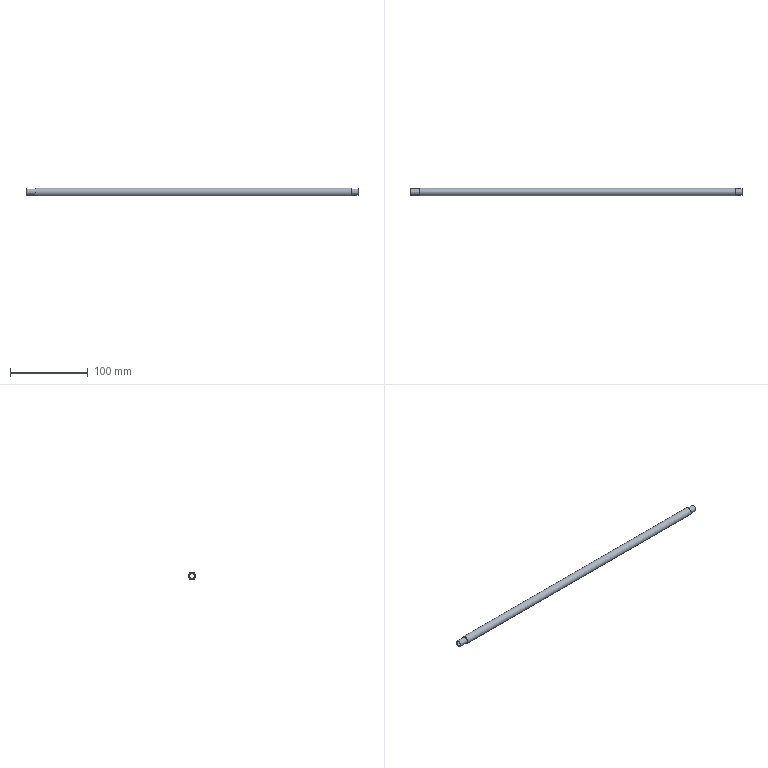Part | STEP file | 1-23.4 | 1 solid | 8 faces | box 427 x 10 x 10 mm | volume 20870 mm3 | cylinder 4 | plane 4 | commonest cylinder face diameters 8 x2 6 x1 10 x1
STEP:
#1=CARTESIAN_POINT('',(0.,0.,0.));
#2=DIRECTION('',(0.,0.,1.));
#3=DIRECTION('',(1.,0.,0.));
#4=AXIS2_PLACEMENT_3D('',#1,#2,#3);
#5=CARTESIAN_POINT('',(0.,5.,0.));
#6=VERTEX_POINT('',#5);
#7=CARTESIAN_POINT('',(-406.,5.,0.));
#8=VERTEX_POINT('',#7);
#9=CARTESIAN_POINT('',(0.,5.,0.));
#10=DIRECTION('',(-1.,0.,0.));
#11=VECTOR('',#10,1.);
#12=LINE('',#9,#11);
#13=CARTESIAN_POINT('',(0.,0.,0.));
#14=DIRECTION('',(-1.,0.,0.));
#15=DIRECTION('',(0.,1.,0.));
#16=AXIS2_PLACEMENT_3D('',#13,#14,#15);
#17=CYLINDRICAL_SURFACE('',#16,5.);
#18=CARTESIAN_POINT('',(6.283,0.));
#19=DIRECTION('',(0.,1.));
#20=VECTOR('',#19,1.);
#21=LINE('',#18,#20);
#22=(GEOMETRIC_REPRESENTATION_CONTEXT(2)PARAMETRIC_REPRESENTATION_CONTEXT()REPRESENTATION_CONTEXT('',''));
#23=DEFINITIONAL_REPRESENTATION('',(#21),#22);
#24=PCURVE('',#17,#23);
#25=CARTESIAN_POINT('',(0.,0.));
#26=DIRECTION('',(0.,1.));
#27=VECTOR('',#26,1.);
#28=LINE('',#25,#27);
#29=(GEOMETRIC_REPRESENTATION_CONTEXT(2)PARAMETRIC_REPRESENTATION_CONTEXT()REPRESENTATION_CONTEXT('',''));
#30=DEFINITIONAL_REPRESENTATION('',(#28),#29);
#31=PCURVE('',#17,#30);
#32=SEAM_CURVE('',#12,(#24,#31),.PCURVE_S1.);
#33=EDGE_CURVE('',#6,#8,#32,.T.);
#34=ORIENTED_EDGE('',*,*,#33,.T.);
#35=CARTESIAN_POINT('',(-406.,0.,0.));
#36=DIRECTION('',(1.,0.,0.));
#37=DIRECTION('',(0.,1.,0.));
#38=AXIS2_PLACEMENT_3D('',#35,#36,#37);
#39=CIRCLE('',#38,5.);
#40=CARTESIAN_POINT('',(6.283,406.));
#41=DIRECTION('',(-1.,0.));
#42=VECTOR('',#41,1.);
#43=LINE('',#40,#42);
#44=(GEOMETRIC_REPRESENTATION_CONTEXT(2)PARAMETRIC_REPRESENTATION_CONTEXT()REPRESENTATION_CONTEXT('',''));
#45=DEFINITIONAL_REPRESENTATION('',(#43),#44);
#46=PCURVE('',#17,#45);
#47=CARTESIAN_POINT('',(-406.,-1.34,0.));
#48=DIRECTION('',(1.,0.,0.));
#49=DIRECTION('',(0.,0.,-1.));
#50=AXIS2_PLACEMENT_3D('',#47,#48,#49);
#51=PLANE('',#50);
#52=CARTESIAN_POINT('',(0.,1.34));
#53=DIRECTION('',(0.,1.));
#54=AXIS2_PLACEMENT_2D('',#52,#53);
#55=CIRCLE('',#54,5.);
#56=(GEOMETRIC_REPRESENTATION_CONTEXT(2)PARAMETRIC_REPRESENTATION_CONTEXT()REPRESENTATION_CONTEXT('',''));
#57=DEFINITIONAL_REPRESENTATION('',(#55),#56);
#58=PCURVE('',#51,#57);
#59=SURFACE_CURVE('',#39,(#46,#58),.PCURVE_S1.);
#60=EDGE_CURVE('',#8,#8,#59,.T.);
#61=ORIENTED_EDGE('',*,*,#60,.T.);
#62=ORIENTED_EDGE('',*,*,#33,.F.);
#63=CARTESIAN_POINT('',(0.,0.,0.));
#64=DIRECTION('',(1.,0.,0.));
#65=DIRECTION('',(0.,1.,0.));
#66=AXIS2_PLACEMENT_3D('',#63,#64,#65);
#67=CIRCLE('',#66,5.);
#68=CARTESIAN_POINT('',(6.283,0.));
#69=DIRECTION('',(-1.,0.));
#70=VECTOR('',#69,1.);
#71=LINE('',#68,#70);
#72=(GEOMETRIC_REPRESENTATION_CONTEXT(2)PARAMETRIC_REPRESENTATION_CONTEXT()REPRESENTATION_CONTEXT('',''));
#73=DEFINITIONAL_REPRESENTATION('',(#71),#72);
#74=PCURVE('',#17,#73);
#75=CARTESIAN_POINT('',(0.,-1.34,0.));
#76=DIRECTION('',(1.,0.,0.));
#77=DIRECTION('',(0.,0.,-1.));
#78=AXIS2_PLACEMENT_3D('',#75,#76,#77);
#79=PLANE('',#78);
#80=CARTESIAN_POINT('',(0.,1.34));
#81=DIRECTION('',(0.,1.));
#82=AXIS2_PLACEMENT_2D('',#80,#81);
#83=CIRCLE('',#82,5.);
#84=(GEOMETRIC_REPRESENTATION_CONTEXT(2)PARAMETRIC_REPRESENTATION_CONTEXT()REPRESENTATION_CONTEXT('',''));
#85=DEFINITIONAL_REPRESENTATION('',(#83),#84);
#86=PCURVE('',#79,#85);
#87=SURFACE_CURVE('',#67,(#74,#86),.PCURVE_S1.);
#88=EDGE_CURVE('',#6,#6,#87,.T.);
#89=ORIENTED_EDGE('',*,*,#88,.F.);
#90=EDGE_LOOP('',(#34,#61,#62,#89));
#91=FACE_BOUND('',#90,.T.);
#92=ADVANCED_FACE('',(#91),#17,.T.);
#93=ORIENTED_EDGE('',*,*,#88,.T.);
#94=EDGE_LOOP('',(#93));
#95=FACE_BOUND('',#94,.T.);
#96=CARTESIAN_POINT('',(0.,4.,0.));
#97=VERTEX_POINT('',#96);
#98=CARTESIAN_POINT('',(0.,0.,0.));
#99=DIRECTION('',(1.,0.,0.));
#100=DIRECTION('',(0.,1.,0.));
#101=AXIS2_PLACEMENT_3D('',#98,#99,#100);
#102=CIRCLE('',#101,4.);
#103=CARTESIAN_POINT('',(0.,1.34));
#104=DIRECTION('',(0.,1.));
#105=AXIS2_PLACEMENT_2D('',#103,#104);
#106=CIRCLE('',#105,4.);
#107=(GEOMETRIC_REPRESENTATION_CONTEXT(2)PARAMETRIC_REPRESENTATION_CONTEXT()REPRESENTATION_CONTEXT('',''));
#108=DEFINITIONAL_REPRESENTATION('',(#106),#107);
#109=PCURVE('',#79,#108);
#110=CARTESIAN_POINT('',(0.,0.,0.));
#111=DIRECTION('',(1.,0.,0.));
#112=DIRECTION('',(0.,1.,0.));
#113=AXIS2_PLACEMENT_3D('',#110,#111,#112);
#114=CYLINDRICAL_SURFACE('',#113,4.);
#115=CARTESIAN_POINT('',(0.,0.));
#116=DIRECTION('',(1.,0.));
#117=VECTOR('',#116,1.);
#118=LINE('',#115,#117);
#119=(GEOMETRIC_REPRESENTATION_CONTEXT(2)PARAMETRIC_REPRESENTATION_CONTEXT()REPRESENTATION_CONTEXT('',''));
#120=DEFINITIONAL_REPRESENTATION('',(#118),#119);
#121=PCURVE('',#114,#120);
#122=SURFACE_CURVE('',#102,(#109,#121),.PCURVE_S1.);
#123=EDGE_CURVE('',#97,#97,#122,.T.);
#124=ORIENTED_EDGE('',*,*,#123,.F.);
#125=EDGE_LOOP('',(#124));
#126=FACE_BOUND('',#125,.T.);
#127=ADVANCED_FACE('',(#95,#126),#79,.T.);
#128=ORIENTED_EDGE('',*,*,#123,.T.);
#129=CARTESIAN_POINT('',(9.,4.,0.));
#130=VERTEX_POINT('',#129);
#131=CARTESIAN_POINT('',(0.,4.,0.));
#132=DIRECTION('',(1.,0.,0.));
#133=VECTOR('',#132,1.);
#134=LINE('',#131,#133);
#135=CARTESIAN_POINT('',(6.283,0.));
#136=DIRECTION('',(0.,1.));
#137=VECTOR('',#136,1.);
#138=LINE('',#135,#137);
#139=(GEOMETRIC_REPRESENTATION_CONTEXT(2)PARAMETRIC_REPRESENTATION_CONTEXT()REPRESENTATION_CONTEXT('',''));
#140=DEFINITIONAL_REPRESENTATION('',(#138),#139);
#141=PCURVE('',#114,#140);
#142=CARTESIAN_POINT('',(0.,0.));
#143=DIRECTION('',(0.,1.));
#144=VECTOR('',#143,1.);
#145=LINE('',#142,#144);
#146=(GEOMETRIC_REPRESENTATION_CONTEXT(2)PARAMETRIC_REPRESENTATION_CONTEXT()REPRESENTATION_CONTEXT('',''));
#147=DEFINITIONAL_REPRESENTATION('',(#145),#146);
#148=PCURVE('',#114,#147);
#149=SEAM_CURVE('',#134,(#141,#148),.PCURVE_S1.);
#150=EDGE_CURVE('',#97,#130,#149,.T.);
#151=ORIENTED_EDGE('',*,*,#150,.T.);
#152=CARTESIAN_POINT('',(9.,0.,0.));
#153=DIRECTION('',(1.,0.,0.));
#154=DIRECTION('',(0.,1.,0.));
#155=AXIS2_PLACEMENT_3D('',#152,#153,#154);
#156=CIRCLE('',#155,4.);
#157=CARTESIAN_POINT('',(0.,9.));
#158=DIRECTION('',(1.,0.));
#159=VECTOR('',#158,1.);
#160=LINE('',#157,#159);
#161=(GEOMETRIC_REPRESENTATION_CONTEXT(2)PARAMETRIC_REPRESENTATION_CONTEXT()REPRESENTATION_CONTEXT('',''));
#162=DEFINITIONAL_REPRESENTATION('',(#160),#161);
#163=PCURVE('',#114,#162);
#164=CARTESIAN_POINT('',(9.,-1.072,0.));
#165=DIRECTION('',(1.,0.,0.));
#166=DIRECTION('',(0.,0.,-1.));
#167=AXIS2_PLACEMENT_3D('',#164,#165,#166);
#168=PLANE('',#167);
#169=CARTESIAN_POINT('',(0.,1.072));
#170=DIRECTION('',(0.,1.));
#171=AXIS2_PLACEMENT_2D('',#169,#170);
#172=CIRCLE('',#171,4.);
#173=(GEOMETRIC_REPRESENTATION_CONTEXT(2)PARAMETRIC_REPRESENTATION_CONTEXT()REPRESENTATION_CONTEXT('',''));
#174=DEFINITIONAL_REPRESENTATION('',(#172),#173);
#175=PCURVE('',#168,#174);
#176=SURFACE_CURVE('',#156,(#163,#175),.PCURVE_S1.);
#177=EDGE_CURVE('',#130,#130,#176,.T.);
#178=ORIENTED_EDGE('',*,*,#177,.F.);
#179=ORIENTED_EDGE('',*,*,#150,.F.);
#180=EDGE_LOOP('',(#128,#151,#178,#179));
#181=FACE_BOUND('',#180,.T.);
#182=ADVANCED_FACE('',(#181),#114,.T.);
#183=ORIENTED_EDGE('',*,*,#60,.T.);
#184=EDGE_LOOP('',(#183));
#185=FACE_BOUND('',#184,.F.);
#186=CARTESIAN_POINT('',(-406.,-4.,0.));
#187=VERTEX_POINT('',#186);
#188=CARTESIAN_POINT('',(-406.,0.,0.));
#189=DIRECTION('',(-1.,0.,0.));
#190=DIRECTION('',(0.,-1.,0.));
#191=AXIS2_PLACEMENT_3D('',#188,#189,#190);
#192=CIRCLE('',#191,4.);
#193=CARTESIAN_POINT('',(0.,-2.66));
#194=CARTESIAN_POINT('',(-6.928,-2.66));
#195=CARTESIAN_POINT('',(-3.464,3.34));
#196=CARTESIAN_POINT('',(0.,9.34));
#197=CARTESIAN_POINT('',(3.464,3.34));
#198=CARTESIAN_POINT('',(6.928,-2.66));
#199=CARTESIAN_POINT('',(0.,-2.66));
#200=(BOUNDED_CURVE()B_SPLINE_CURVE(2,(#193,#194,#195,#196,#197,#198,#199),.UNSPECIFIED.,.T.,.F.)B_SPLINE_CURVE_WITH_KNOTS((1,2,2,2,2,1),(-2.094,0.,2.094,4.189,6.283,8.378),.UNSPECIFIED.)CURVE()GEOMETRIC_REPRESENTATION_ITEM()RATIONAL_B_SPLINE_CURVE((1.,0.5,1.,0.5,1.,0.5,1.))REPRESENTATION_ITEM(''));
#201=(GEOMETRIC_REPRESENTATION_CONTEXT(2)PARAMETRIC_REPRESENTATION_CONTEXT()REPRESENTATION_CONTEXT('',''));
#202=DEFINITIONAL_REPRESENTATION('',(#200),#201);
#203=PCURVE('',#51,#202);
#204=CARTESIAN_POINT('',(-406.,0.,0.));
#205=DIRECTION('',(-1.,0.,0.));
#206=DIRECTION('',(0.,-1.,0.));
#207=AXIS2_PLACEMENT_3D('',#204,#205,#206);
#208=CYLINDRICAL_SURFACE('',#207,4.);
#209=CARTESIAN_POINT('',(0.,0.));
#210=DIRECTION('',(1.,0.));
#211=VECTOR('',#210,1.);
#212=LINE('',#209,#211);
#213=(GEOMETRIC_REPRESENTATION_CONTEXT(2)PARAMETRIC_REPRESENTATION_CONTEXT()REPRESENTATION_CONTEXT('',''));
#214=DEFINITIONAL_REPRESENTATION('',(#212),#213);
#215=PCURVE('',#208,#214);
#216=SURFACE_CURVE('',#192,(#203,#215),.PCURVE_S1.);
#217=EDGE_CURVE('',#187,#187,#216,.T.);
#218=ORIENTED_EDGE('',*,*,#217,.T.);
#219=EDGE_LOOP('',(#218));
#220=FACE_BOUND('',#219,.F.);
#221=ADVANCED_FACE('',(#185,#220),#51,.F.);
#222=ORIENTED_EDGE('',*,*,#217,.T.);
#223=CARTESIAN_POINT('',(-418.,-4.,0.));
#224=VERTEX_POINT('',#223);
#225=CARTESIAN_POINT('',(-406.,-4.,0.));
#226=DIRECTION('',(-1.,0.,0.));
#227=VECTOR('',#226,1.);
#228=LINE('',#225,#227);
#229=CARTESIAN_POINT('',(6.283,0.));
#230=DIRECTION('',(0.,1.));
#231=VECTOR('',#230,1.);
#232=LINE('',#229,#231);
#233=(GEOMETRIC_REPRESENTATION_CONTEXT(2)PARAMETRIC_REPRESENTATION_CONTEXT()REPRESENTATION_CONTEXT('',''));
#234=DEFINITIONAL_REPRESENTATION('',(#232),#233);
#235=PCURVE('',#208,#234);
#236=CARTESIAN_POINT('',(0.,0.));
#237=DIRECTION('',(0.,1.));
#238=VECTOR('',#237,1.);
#239=LINE('',#236,#238);
#240=(GEOMETRIC_REPRESENTATION_CONTEXT(2)PARAMETRIC_REPRESENTATION_CONTEXT()REPRESENTATION_CONTEXT('',''));
#241=DEFINITIONAL_REPRESENTATION('',(#239),#240);
#242=PCURVE('',#208,#241);
#243=SEAM_CURVE('',#228,(#235,#242),.PCURVE_S1.);
#244=EDGE_CURVE('',#187,#224,#243,.T.);
#245=ORIENTED_EDGE('',*,*,#244,.T.);
#246=CARTESIAN_POINT('',(-418.,0.,0.));
#247=DIRECTION('',(-1.,0.,0.));
#248=DIRECTION('',(0.,-1.,0.));
#249=AXIS2_PLACEMENT_3D('',#246,#247,#248);
#250=CIRCLE('',#249,4.);
#251=CARTESIAN_POINT('',(0.,12.));
#252=DIRECTION('',(1.,0.));
#253=VECTOR('',#252,1.);
#254=LINE('',#251,#253);
#255=(GEOMETRIC_REPRESENTATION_CONTEXT(2)PARAMETRIC_REPRESENTATION_CONTEXT()REPRESENTATION_CONTEXT('',''));
#256=DEFINITIONAL_REPRESENTATION('',(#254),#255);
#257=PCURVE('',#208,#256);
#258=CARTESIAN_POINT('',(-418.,1.072,0.));
#259=DIRECTION('',(-1.,0.,0.));
#260=DIRECTION('',(0.,-1.,0.));
#261=AXIS2_PLACEMENT_3D('',#258,#259,#260);
#262=PLANE('',#261);
#263=CARTESIAN_POINT('',(1.072,0.));
#264=DIRECTION('',(1.,0.));
#265=AXIS2_PLACEMENT_2D('',#263,#264);
#266=CIRCLE('',#265,4.);
#267=(GEOMETRIC_REPRESENTATION_CONTEXT(2)PARAMETRIC_REPRESENTATION_CONTEXT()REPRESENTATION_CONTEXT('',''));
#268=DEFINITIONAL_REPRESENTATION('',(#266),#267);
#269=PCURVE('',#262,#268);
#270=SURFACE_CURVE('',#250,(#257,#269),.PCURVE_S1.);
#271=EDGE_CURVE('',#224,#224,#270,.T.);
#272=ORIENTED_EDGE('',*,*,#271,.F.);
#273=ORIENTED_EDGE('',*,*,#244,.F.);
#274=EDGE_LOOP('',(#222,#245,#272,#273));
#275=FACE_BOUND('',#274,.T.);
#276=ADVANCED_FACE('',(#275),#208,.T.);
#277=ORIENTED_EDGE('',*,*,#177,.T.);
#278=EDGE_LOOP('',(#277));
#279=FACE_BOUND('',#278,.T.);
#280=CARTESIAN_POINT('',(9.,-3.,0.));
#281=VERTEX_POINT('',#280);
#282=CARTESIAN_POINT('',(9.,0.,0.));
#283=DIRECTION('',(1.,0.,0.));
#284=DIRECTION('',(0.,-1.,0.));
#285=AXIS2_PLACEMENT_3D('',#282,#283,#284);
#286=CIRCLE('',#285,3.);
#287=CARTESIAN_POINT('',(0.,1.072));
#288=DIRECTION('',(0.,-1.));
#289=AXIS2_PLACEMENT_2D('',#287,#288);
#290=CIRCLE('',#289,3.);
#291=(GEOMETRIC_REPRESENTATION_CONTEXT(2)PARAMETRIC_REPRESENTATION_CONTEXT()REPRESENTATION_CONTEXT('',''));
#292=DEFINITIONAL_REPRESENTATION('',(#290),#291);
#293=PCURVE('',#168,#292);
#294=CARTESIAN_POINT('',(-418.,0.,0.));
#295=DIRECTION('',(1.,0.,0.));
#296=DIRECTION('',(0.,-1.,0.));
#297=AXIS2_PLACEMENT_3D('',#294,#295,#296);
#298=CYLINDRICAL_SURFACE('',#297,3.);
#299=CARTESIAN_POINT('',(0.,427.));
#300=DIRECTION('',(1.,0.));
#301=VECTOR('',#300,1.);
#302=LINE('',#299,#301);
#303=(GEOMETRIC_REPRESENTATION_CONTEXT(2)PARAMETRIC_REPRESENTATION_CONTEXT()REPRESENTATION_CONTEXT('',''));
#304=DEFINITIONAL_REPRESENTATION('',(#302),#303);
#305=PCURVE('',#298,#304);
#306=SURFACE_CURVE('',#286,(#293,#305),.PCURVE_S1.);
#307=EDGE_CURVE('',#281,#281,#306,.T.);
#308=ORIENTED_EDGE('',*,*,#307,.F.);
#309=EDGE_LOOP('',(#308));
#310=FACE_BOUND('',#309,.T.);
#311=ADVANCED_FACE('',(#279,#310),#168,.T.);
#312=ORIENTED_EDGE('',*,*,#271,.T.);
#313=EDGE_LOOP('',(#312));
#314=FACE_BOUND('',#313,.T.);
#315=CARTESIAN_POINT('',(-418.,-3.,0.));
#316=VERTEX_POINT('',#315);
#317=CARTESIAN_POINT('',(-418.,0.,0.));
#318=DIRECTION('',(-1.,0.,0.));
#319=DIRECTION('',(0.,-1.,0.));
#320=AXIS2_PLACEMENT_3D('',#317,#318,#319);
#321=CIRCLE('',#320,3.);
#322=CARTESIAN_POINT('',(1.072,0.));
#323=DIRECTION('',(1.,0.));
#324=AXIS2_PLACEMENT_2D('',#322,#323);
#325=CIRCLE('',#324,3.);
#326=(GEOMETRIC_REPRESENTATION_CONTEXT(2)PARAMETRIC_REPRESENTATION_CONTEXT()REPRESENTATION_CONTEXT('',''));
#327=DEFINITIONAL_REPRESENTATION('',(#325),#326);
#328=PCURVE('',#262,#327);
#329=CARTESIAN_POINT('',(6.283,0.));
#330=DIRECTION('',(-1.,0.));
#331=VECTOR('',#330,1.);
#332=LINE('',#329,#331);
#333=(GEOMETRIC_REPRESENTATION_CONTEXT(2)PARAMETRIC_REPRESENTATION_CONTEXT()REPRESENTATION_CONTEXT('',''));
#334=DEFINITIONAL_REPRESENTATION('',(#332),#333);
#335=PCURVE('',#298,#334);
#336=SURFACE_CURVE('',#321,(#328,#335),.PCURVE_S1.);
#337=EDGE_CURVE('',#316,#316,#336,.T.);
#338=ORIENTED_EDGE('',*,*,#337,.F.);
#339=EDGE_LOOP('',(#338));
#340=FACE_BOUND('',#339,.T.);
#341=ADVANCED_FACE('',(#314,#340),#262,.T.);
#342=CARTESIAN_POINT('',(-418.,-3.,0.));
#343=DIRECTION('',(1.,0.,0.));
#344=VECTOR('',#343,1.);
#345=LINE('',#342,#344);
#346=CARTESIAN_POINT('',(6.283,0.));
#347=DIRECTION('',(0.,1.));
#348=VECTOR('',#347,1.);
#349=LINE('',#346,#348);
#350=(GEOMETRIC_REPRESENTATION_CONTEXT(2)PARAMETRIC_REPRESENTATION_CONTEXT()REPRESENTATION_CONTEXT('',''));
#351=DEFINITIONAL_REPRESENTATION('',(#349),#350);
#352=PCURVE('',#298,#351);
#353=CARTESIAN_POINT('',(0.,0.));
#354=DIRECTION('',(0.,1.));
#355=VECTOR('',#354,1.);
#356=LINE('',#353,#355);
#357=(GEOMETRIC_REPRESENTATION_CONTEXT(2)PARAMETRIC_REPRESENTATION_CONTEXT()REPRESENTATION_CONTEXT('',''));
#358=DEFINITIONAL_REPRESENTATION('',(#356),#357);
#359=PCURVE('',#298,#358);
#360=SEAM_CURVE('',#345,(#352,#359),.PCURVE_S1.);
#361=EDGE_CURVE('',#316,#281,#360,.T.);
#362=ORIENTED_EDGE('',*,*,#361,.T.);
#363=ORIENTED_EDGE('',*,*,#307,.F.);
#364=ORIENTED_EDGE('',*,*,#361,.F.);
#365=ORIENTED_EDGE('',*,*,#337,.F.);
#366=EDGE_LOOP('',(#362,#363,#364,#365));
#367=FACE_BOUND('',#366,.F.);
#368=ADVANCED_FACE('',(#367),#298,.F.);
#369=CLOSED_SHELL('',(#92,#127,#182,#221,#276,#311,#341,#368));
#370=MANIFOLD_SOLID_BREP('',#369);
#371=(LENGTH_UNIT()NAMED_UNIT(*)SI_UNIT(.MILLI.,.METRE.));
#372=UNCERTAINTY_MEASURE_WITH_UNIT(LENGTH_MEASURE(0.0000001),#371,'','');
#373=(NAMED_UNIT(*)PLANE_ANGLE_UNIT()SI_UNIT($,.RADIAN.));
#374=(NAMED_UNIT(*)SI_UNIT($,.STERADIAN.)SOLID_ANGLE_UNIT());
#375=(GEOMETRIC_REPRESENTATION_CONTEXT(3)GLOBAL_UNCERTAINTY_ASSIGNED_CONTEXT((#372))GLOBAL_UNIT_ASSIGNED_CONTEXT((#371,#373,#374))REPRESENTATION_CONTEXT('',''));
#376=ADVANCED_BREP_SHAPE_REPRESENTATION('',(#4,#370),#375);